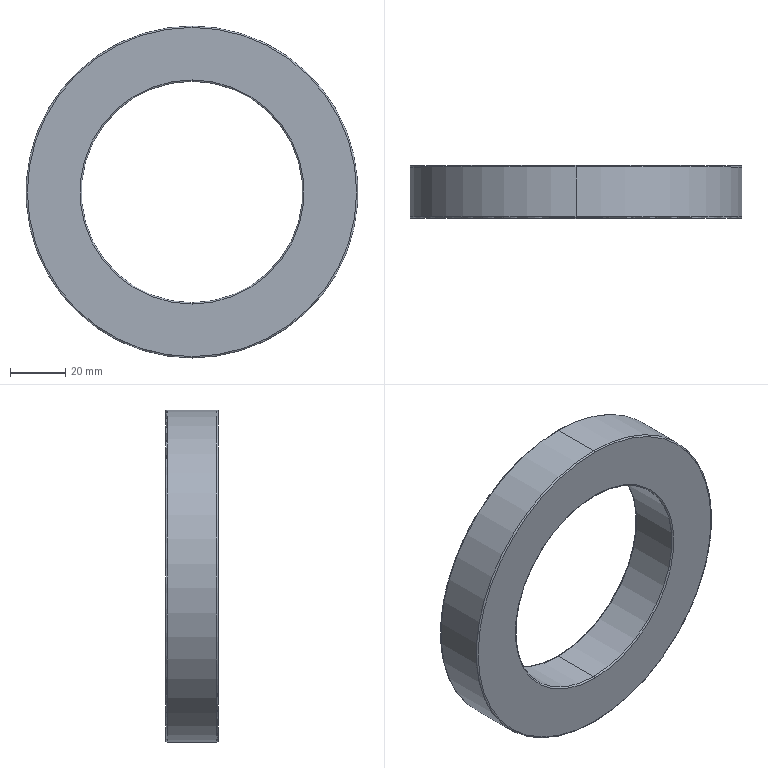Part | STEP file | 2026.6.15-Main Assembly图.sldasm-Part-126 | 1 solid | 14 faces | box 120 x 19 x 120 mm | volume 119313 mm3 | torus 8 | cylinder 4 | plane 2 | commonest cylinder face diameters 80 x2 120 x2
STEP:
#1=CARTESIAN_POINT('',(-1589.224,623.551,4168.167));
#2=VERTEX_POINT('',#1);
#3=CARTESIAN_POINT('',(-1589.224,623.551,4249.167));
#4=VERTEX_POINT('',#3);
#5=CARTESIAN_POINT('',(-1589.224,623.551,4208.667));
#6=DIRECTION('',(0.,-1.,0.));
#7=DIRECTION('',(0.,0.,1.));
#8=AXIS2_PLACEMENT_3D('',#5,#6,#7);
#9=CIRCLE('',#8,40.5);
#10=EDGE_CURVE('',#2,#4,#9,.T.);
#11=ORIENTED_EDGE('',*,*,#10,.F.);
#12=CARTESIAN_POINT('',(-1589.224,623.051,4168.667));
#13=VERTEX_POINT('',#12);
#14=CARTESIAN_POINT('',(-1589.224,623.051,4168.167));
#15=DIRECTION('',(1.,0.,0.));
#16=DIRECTION('',(0.,0.,-1.));
#17=AXIS2_PLACEMENT_3D('',#14,#15,#16);
#18=CIRCLE('',#17,0.5);
#19=EDGE_CURVE('',#2,#13,#18,.T.);
#20=ORIENTED_EDGE('',*,*,#19,.T.);
#21=CARTESIAN_POINT('',(-1589.224,623.051,4248.667));
#22=VERTEX_POINT('',#21);
#23=CARTESIAN_POINT('',(-1589.224,623.051,4208.667));
#24=DIRECTION('',(0.,1.,0.));
#25=DIRECTION('',(0.,0.,1.));
#26=AXIS2_PLACEMENT_3D('',#23,#24,#25);
#27=CIRCLE('',#26,40.);
#28=EDGE_CURVE('',#22,#13,#27,.T.);
#29=ORIENTED_EDGE('',*,*,#28,.F.);
#30=CARTESIAN_POINT('',(-1589.224,623.051,4249.167));
#31=DIRECTION('',(-1.,0.,0.));
#32=DIRECTION('',(0.,0.,1.));
#33=AXIS2_PLACEMENT_3D('',#30,#31,#32);
#34=CIRCLE('',#33,0.5);
#35=EDGE_CURVE('',#4,#22,#34,.T.);
#36=ORIENTED_EDGE('',*,*,#35,.F.);
#37=EDGE_LOOP('',(#11,#20,#29,#36));
#38=FACE_OUTER_BOUND('',#37,.T.);
#39=CARTESIAN_POINT('',(-1589.224,623.051,4208.667));
#40=DIRECTION('',(0.,1.,0.));
#41=DIRECTION('',(0.,0.,1.));
#42=AXIS2_PLACEMENT_3D('',#39,#40,#41);
#43=TOROIDAL_SURFACE('',#42,40.5,0.5);
#44=ADVANCED_FACE('',(#38),#43,.T.);
#45=CARTESIAN_POINT('',(-1589.224,623.051,4148.667));
#46=VERTEX_POINT('',#45);
#47=CARTESIAN_POINT('',(-1589.224,623.051,4268.667));
#48=VERTEX_POINT('',#47);
#49=CARTESIAN_POINT('',(-1589.224,623.051,4208.667));
#50=DIRECTION('',(0.,-1.,0.));
#51=DIRECTION('',(0.,0.,1.));
#52=AXIS2_PLACEMENT_3D('',#49,#50,#51);
#53=CIRCLE('',#52,60.);
#54=EDGE_CURVE('',#46,#48,#53,.T.);
#55=ORIENTED_EDGE('',*,*,#54,.F.);
#56=CARTESIAN_POINT('',(-1589.224,623.551,4149.167));
#57=VERTEX_POINT('',#56);
#58=CARTESIAN_POINT('',(-1589.224,623.051,4149.167));
#59=DIRECTION('',(1.,0.,0.));
#60=DIRECTION('',(0.,0.,-1.));
#61=AXIS2_PLACEMENT_3D('',#58,#59,#60);
#62=CIRCLE('',#61,0.5);
#63=EDGE_CURVE('',#46,#57,#62,.T.);
#64=ORIENTED_EDGE('',*,*,#63,.T.);
#65=CARTESIAN_POINT('',(-1589.224,623.551,4268.167));
#66=VERTEX_POINT('',#65);
#67=CARTESIAN_POINT('',(-1589.224,623.551,4208.667));
#68=DIRECTION('',(0.,1.,0.));
#69=DIRECTION('',(0.,0.,1.));
#70=AXIS2_PLACEMENT_3D('',#67,#68,#69);
#71=CIRCLE('',#70,59.5);
#72=EDGE_CURVE('',#66,#57,#71,.T.);
#73=ORIENTED_EDGE('',*,*,#72,.F.);
#74=CARTESIAN_POINT('',(-1589.224,623.051,4268.167));
#75=DIRECTION('',(-1.,0.,0.));
#76=DIRECTION('',(0.,0.,1.));
#77=AXIS2_PLACEMENT_3D('',#74,#75,#76);
#78=CIRCLE('',#77,0.5);
#79=EDGE_CURVE('',#48,#66,#78,.T.);
#80=ORIENTED_EDGE('',*,*,#79,.F.);
#81=EDGE_LOOP('',(#55,#64,#73,#80));
#82=FACE_OUTER_BOUND('',#81,.T.);
#83=CARTESIAN_POINT('',(-1589.224,623.051,4208.667));
#84=DIRECTION('',(0.,1.,0.));
#85=DIRECTION('',(0.,0.,1.));
#86=AXIS2_PLACEMENT_3D('',#83,#84,#85);
#87=TOROIDAL_SURFACE('',#86,59.5,0.5);
#88=ADVANCED_FACE('',(#82),#87,.T.);
#89=CARTESIAN_POINT('',(-1589.224,604.551,4249.167));
#90=VERTEX_POINT('',#89);
#91=CARTESIAN_POINT('',(-1589.224,604.551,4168.167));
#92=VERTEX_POINT('',#91);
#93=CARTESIAN_POINT('',(-1589.224,604.551,4208.667));
#94=DIRECTION('',(0.,1.,0.));
#95=DIRECTION('',(0.,0.,-1.));
#96=AXIS2_PLACEMENT_3D('',#93,#94,#95);
#97=CIRCLE('',#96,40.5);
#98=EDGE_CURVE('',#90,#92,#97,.T.);
#99=ORIENTED_EDGE('',*,*,#98,.F.);
#100=CARTESIAN_POINT('',(-1589.224,605.051,4248.667));
#101=VERTEX_POINT('',#100);
#102=CARTESIAN_POINT('',(-1589.224,605.051,4249.167));
#103=DIRECTION('',(1.,0.,0.));
#104=DIRECTION('',(0.,0.,-1.));
#105=AXIS2_PLACEMENT_3D('',#102,#103,#104);
#106=CIRCLE('',#105,0.5);
#107=EDGE_CURVE('',#90,#101,#106,.T.);
#108=ORIENTED_EDGE('',*,*,#107,.T.);
#109=CARTESIAN_POINT('',(-1589.224,605.051,4168.667));
#110=VERTEX_POINT('',#109);
#111=CARTESIAN_POINT('',(-1589.224,605.051,4208.667));
#112=DIRECTION('',(0.,-1.,0.));
#113=DIRECTION('',(0.,0.,-1.));
#114=AXIS2_PLACEMENT_3D('',#111,#112,#113);
#115=CIRCLE('',#114,40.);
#116=EDGE_CURVE('',#110,#101,#115,.T.);
#117=ORIENTED_EDGE('',*,*,#116,.F.);
#118=CARTESIAN_POINT('',(-1589.224,605.051,4168.167));
#119=DIRECTION('',(-1.,0.,0.));
#120=DIRECTION('',(0.,0.,1.));
#121=AXIS2_PLACEMENT_3D('',#118,#119,#120);
#122=CIRCLE('',#121,0.5);
#123=EDGE_CURVE('',#92,#110,#122,.T.);
#124=ORIENTED_EDGE('',*,*,#123,.F.);
#125=EDGE_LOOP('',(#99,#108,#117,#124));
#126=FACE_OUTER_BOUND('',#125,.T.);
#127=CARTESIAN_POINT('',(-1589.224,605.051,4208.667));
#128=DIRECTION('',(0.,-1.,0.));
#129=DIRECTION('',(0.,0.,-1.));
#130=AXIS2_PLACEMENT_3D('',#127,#128,#129);
#131=TOROIDAL_SURFACE('',#130,40.5,0.5);
#132=ADVANCED_FACE('',(#126),#131,.T.);
#133=CARTESIAN_POINT('',(-1589.224,605.051,4268.667));
#134=VERTEX_POINT('',#133);
#135=CARTESIAN_POINT('',(-1589.224,605.051,4148.667));
#136=VERTEX_POINT('',#135);
#137=CARTESIAN_POINT('',(-1589.224,605.051,4208.667));
#138=DIRECTION('',(0.,1.,0.));
#139=DIRECTION('',(0.,0.,-1.));
#140=AXIS2_PLACEMENT_3D('',#137,#138,#139);
#141=CIRCLE('',#140,60.);
#142=EDGE_CURVE('',#134,#136,#141,.T.);
#143=ORIENTED_EDGE('',*,*,#142,.F.);
#144=CARTESIAN_POINT('',(-1589.224,604.551,4268.167));
#145=VERTEX_POINT('',#144);
#146=CARTESIAN_POINT('',(-1589.224,605.051,4268.167));
#147=DIRECTION('',(1.,0.,0.));
#148=DIRECTION('',(0.,0.,-1.));
#149=AXIS2_PLACEMENT_3D('',#146,#147,#148);
#150=CIRCLE('',#149,0.5);
#151=EDGE_CURVE('',#134,#145,#150,.T.);
#152=ORIENTED_EDGE('',*,*,#151,.T.);
#153=CARTESIAN_POINT('',(-1589.224,604.551,4149.167));
#154=VERTEX_POINT('',#153);
#155=CARTESIAN_POINT('',(-1589.224,604.551,4208.667));
#156=DIRECTION('',(0.,-1.,0.));
#157=DIRECTION('',(0.,0.,-1.));
#158=AXIS2_PLACEMENT_3D('',#155,#156,#157);
#159=CIRCLE('',#158,59.5);
#160=EDGE_CURVE('',#154,#145,#159,.T.);
#161=ORIENTED_EDGE('',*,*,#160,.F.);
#162=CARTESIAN_POINT('',(-1589.224,605.051,4149.167));
#163=DIRECTION('',(-1.,0.,0.));
#164=DIRECTION('',(0.,0.,1.));
#165=AXIS2_PLACEMENT_3D('',#162,#163,#164);
#166=CIRCLE('',#165,0.5);
#167=EDGE_CURVE('',#136,#154,#166,.T.);
#168=ORIENTED_EDGE('',*,*,#167,.F.);
#169=EDGE_LOOP('',(#143,#152,#161,#168));
#170=FACE_OUTER_BOUND('',#169,.T.);
#171=CARTESIAN_POINT('',(-1589.224,605.051,4208.667));
#172=DIRECTION('',(0.,-1.,0.));
#173=DIRECTION('',(0.,0.,-1.));
#174=AXIS2_PLACEMENT_3D('',#171,#172,#173);
#175=TOROIDAL_SURFACE('',#174,59.5,0.5);
#176=ADVANCED_FACE('',(#170),#175,.T.);
#177=CARTESIAN_POINT('',(-1589.224,623.051,4208.667));
#178=DIRECTION('',(0.,1.,0.));
#179=DIRECTION('',(0.,0.,1.));
#180=AXIS2_PLACEMENT_3D('',#177,#178,#179);
#181=CIRCLE('',#180,40.);
#182=EDGE_CURVE('',#13,#22,#181,.T.);
#183=ORIENTED_EDGE('',*,*,#182,.T.);
#184=CARTESIAN_POINT('',(-1589.224,623.551,4248.667));
#185=DIRECTION('',(0.,-1.,0.));
#186=VECTOR('',#185,1000.);
#187=LINE('',#184,#186);
#188=EDGE_CURVE('',#22,#101,#187,.T.);
#189=ORIENTED_EDGE('',*,*,#188,.T.);
#190=CARTESIAN_POINT('',(-1589.224,605.051,4208.667));
#191=DIRECTION('',(0.,-1.,0.));
#192=DIRECTION('',(0.,0.,-1.));
#193=AXIS2_PLACEMENT_3D('',#190,#191,#192);
#194=CIRCLE('',#193,40.);
#195=EDGE_CURVE('',#101,#110,#194,.T.);
#196=ORIENTED_EDGE('',*,*,#195,.T.);
#197=CARTESIAN_POINT('',(-1589.224,623.551,4168.667));
#198=DIRECTION('',(0.,-1.,0.));
#199=VECTOR('',#198,1000.);
#200=LINE('',#197,#199);
#201=EDGE_CURVE('',#13,#110,#200,.T.);
#202=ORIENTED_EDGE('',*,*,#201,.F.);
#203=EDGE_LOOP('',(#183,#189,#196,#202));
#204=FACE_OUTER_BOUND('',#203,.T.);
#205=CARTESIAN_POINT('',(-1589.224,623.551,4208.667));
#206=DIRECTION('',(0.,-1.,0.));
#207=DIRECTION('',(0.,0.,-1.));
#208=AXIS2_PLACEMENT_3D('',#205,#206,#207);
#209=CYLINDRICAL_SURFACE('',#208,40.);
#210=ADVANCED_FACE('',(#204),#209,.F.);
#211=ORIENTED_EDGE('',*,*,#142,.T.);
#212=CARTESIAN_POINT('',(-1589.224,604.551,4148.667));
#213=DIRECTION('',(0.,1.,0.));
#214=VECTOR('',#213,1000.);
#215=LINE('',#212,#214);
#216=EDGE_CURVE('',#136,#46,#215,.T.);
#217=ORIENTED_EDGE('',*,*,#216,.T.);
#218=ORIENTED_EDGE('',*,*,#54,.T.);
#219=CARTESIAN_POINT('',(-1589.224,604.551,4268.667));
#220=DIRECTION('',(0.,1.,0.));
#221=VECTOR('',#220,1000.);
#222=LINE('',#219,#221);
#223=EDGE_CURVE('',#134,#48,#222,.T.);
#224=ORIENTED_EDGE('',*,*,#223,.F.);
#225=EDGE_LOOP('',(#211,#217,#218,#224));
#226=FACE_OUTER_BOUND('',#225,.T.);
#227=CARTESIAN_POINT('',(-1589.224,604.551,4208.667));
#228=DIRECTION('',(0.,1.,0.));
#229=DIRECTION('',(0.,0.,1.));
#230=AXIS2_PLACEMENT_3D('',#227,#228,#229);
#231=CYLINDRICAL_SURFACE('',#230,60.);
#232=ADVANCED_FACE('',(#226),#231,.T.);
#233=ORIENTED_EDGE('',*,*,#72,.T.);
#234=CARTESIAN_POINT('',(-1589.224,623.551,4208.667));
#235=DIRECTION('',(0.,1.,0.));
#236=DIRECTION('',(0.,0.,1.));
#237=AXIS2_PLACEMENT_3D('',#234,#235,#236);
#238=CIRCLE('',#237,59.5);
#239=EDGE_CURVE('',#57,#66,#238,.T.);
#240=ORIENTED_EDGE('',*,*,#239,.T.);
#241=EDGE_LOOP('',(#233,#240));
#242=FACE_OUTER_BOUND('',#241,.T.);
#243=CARTESIAN_POINT('',(-1589.224,623.551,4208.667));
#244=DIRECTION('',(0.,-1.,0.));
#245=DIRECTION('',(0.,0.,1.));
#246=AXIS2_PLACEMENT_3D('',#243,#244,#245);
#247=CIRCLE('',#246,40.5);
#248=EDGE_CURVE('',#4,#2,#247,.T.);
#249=ORIENTED_EDGE('',*,*,#248,.T.);
#250=ORIENTED_EDGE('',*,*,#10,.T.);
#251=EDGE_LOOP('',(#249,#250));
#252=FACE_BOUND('',#251,.T.);
#253=CARTESIAN_POINT('',(-1589.224,623.551,4208.667));
#254=DIRECTION('',(0.,1.,0.));
#255=DIRECTION('',(0.,0.,1.));
#256=AXIS2_PLACEMENT_3D('',#253,#254,#255);
#257=PLANE('',#256);
#258=ADVANCED_FACE('',(#242,#252),#257,.T.);
#259=ORIENTED_EDGE('',*,*,#160,.T.);
#260=CARTESIAN_POINT('',(-1589.224,604.551,4208.667));
#261=DIRECTION('',(0.,-1.,0.));
#262=DIRECTION('',(0.,0.,-1.));
#263=AXIS2_PLACEMENT_3D('',#260,#261,#262);
#264=CIRCLE('',#263,59.5);
#265=EDGE_CURVE('',#145,#154,#264,.T.);
#266=ORIENTED_EDGE('',*,*,#265,.T.);
#267=EDGE_LOOP('',(#259,#266));
#268=FACE_OUTER_BOUND('',#267,.T.);
#269=CARTESIAN_POINT('',(-1589.224,604.551,4208.667));
#270=DIRECTION('',(0.,1.,0.));
#271=DIRECTION('',(0.,0.,-1.));
#272=AXIS2_PLACEMENT_3D('',#269,#270,#271);
#273=CIRCLE('',#272,40.5);
#274=EDGE_CURVE('',#92,#90,#273,.T.);
#275=ORIENTED_EDGE('',*,*,#274,.T.);
#276=ORIENTED_EDGE('',*,*,#98,.T.);
#277=EDGE_LOOP('',(#275,#276));
#278=FACE_BOUND('',#277,.T.);
#279=CARTESIAN_POINT('',(-1589.224,604.551,4208.667));
#280=DIRECTION('',(0.,-1.,0.));
#281=DIRECTION('',(0.,0.,-1.));
#282=AXIS2_PLACEMENT_3D('',#279,#280,#281);
#283=PLANE('',#282);
#284=ADVANCED_FACE('',(#268,#278),#283,.T.);
#285=ORIENTED_EDGE('',*,*,#216,.F.);
#286=CARTESIAN_POINT('',(-1589.224,605.051,4208.667));
#287=DIRECTION('',(0.,1.,0.));
#288=DIRECTION('',(0.,0.,-1.));
#289=AXIS2_PLACEMENT_3D('',#286,#287,#288);
#290=CIRCLE('',#289,60.);
#291=EDGE_CURVE('',#136,#134,#290,.T.);
#292=ORIENTED_EDGE('',*,*,#291,.T.);
#293=ORIENTED_EDGE('',*,*,#223,.T.);
#294=CARTESIAN_POINT('',(-1589.224,623.051,4208.667));
#295=DIRECTION('',(0.,-1.,0.));
#296=DIRECTION('',(0.,0.,1.));
#297=AXIS2_PLACEMENT_3D('',#294,#295,#296);
#298=CIRCLE('',#297,60.);
#299=EDGE_CURVE('',#48,#46,#298,.T.);
#300=ORIENTED_EDGE('',*,*,#299,.T.);
#301=EDGE_LOOP('',(#285,#292,#293,#300));
#302=FACE_OUTER_BOUND('',#301,.T.);
#303=CARTESIAN_POINT('',(-1589.224,604.551,4208.667));
#304=DIRECTION('',(0.,1.,0.));
#305=DIRECTION('',(0.,0.,1.));
#306=AXIS2_PLACEMENT_3D('',#303,#304,#305);
#307=CYLINDRICAL_SURFACE('',#306,60.);
#308=ADVANCED_FACE('',(#302),#307,.T.);
#309=ORIENTED_EDGE('',*,*,#188,.F.);
#310=ORIENTED_EDGE('',*,*,#28,.T.);
#311=ORIENTED_EDGE('',*,*,#201,.T.);
#312=ORIENTED_EDGE('',*,*,#116,.T.);
#313=EDGE_LOOP('',(#309,#310,#311,#312));
#314=FACE_OUTER_BOUND('',#313,.T.);
#315=CARTESIAN_POINT('',(-1589.224,623.551,4208.667));
#316=DIRECTION('',(0.,-1.,0.));
#317=DIRECTION('',(0.,0.,-1.));
#318=AXIS2_PLACEMENT_3D('',#315,#316,#317);
#319=CYLINDRICAL_SURFACE('',#318,40.);
#320=ADVANCED_FACE('',(#314),#319,.F.);
#321=ORIENTED_EDGE('',*,*,#151,.F.);
#322=ORIENTED_EDGE('',*,*,#291,.F.);
#323=ORIENTED_EDGE('',*,*,#167,.T.);
#324=ORIENTED_EDGE('',*,*,#265,.F.);
#325=EDGE_LOOP('',(#321,#322,#323,#324));
#326=FACE_OUTER_BOUND('',#325,.T.);
#327=CARTESIAN_POINT('',(-1589.224,605.051,4208.667));
#328=DIRECTION('',(0.,-1.,0.));
#329=DIRECTION('',(0.,0.,-1.));
#330=AXIS2_PLACEMENT_3D('',#327,#328,#329);
#331=TOROIDAL_SURFACE('',#330,59.5,0.5);
#332=ADVANCED_FACE('',(#326),#331,.T.);
#333=ORIENTED_EDGE('',*,*,#107,.F.);
#334=ORIENTED_EDGE('',*,*,#274,.F.);
#335=ORIENTED_EDGE('',*,*,#123,.T.);
#336=ORIENTED_EDGE('',*,*,#195,.F.);
#337=EDGE_LOOP('',(#333,#334,#335,#336));
#338=FACE_OUTER_BOUND('',#337,.T.);
#339=CARTESIAN_POINT('',(-1589.224,605.051,4208.667));
#340=DIRECTION('',(0.,-1.,0.));
#341=DIRECTION('',(0.,0.,-1.));
#342=AXIS2_PLACEMENT_3D('',#339,#340,#341);
#343=TOROIDAL_SURFACE('',#342,40.5,0.5);
#344=ADVANCED_FACE('',(#338),#343,.T.);
#345=ORIENTED_EDGE('',*,*,#63,.F.);
#346=ORIENTED_EDGE('',*,*,#299,.F.);
#347=ORIENTED_EDGE('',*,*,#79,.T.);
#348=ORIENTED_EDGE('',*,*,#239,.F.);
#349=EDGE_LOOP('',(#345,#346,#347,#348));
#350=FACE_OUTER_BOUND('',#349,.T.);
#351=CARTESIAN_POINT('',(-1589.224,623.051,4208.667));
#352=DIRECTION('',(0.,1.,0.));
#353=DIRECTION('',(0.,0.,1.));
#354=AXIS2_PLACEMENT_3D('',#351,#352,#353);
#355=TOROIDAL_SURFACE('',#354,59.5,0.5);
#356=ADVANCED_FACE('',(#350),#355,.T.);
#357=ORIENTED_EDGE('',*,*,#19,.F.);
#358=ORIENTED_EDGE('',*,*,#248,.F.);
#359=ORIENTED_EDGE('',*,*,#35,.T.);
#360=ORIENTED_EDGE('',*,*,#182,.F.);
#361=EDGE_LOOP('',(#357,#358,#359,#360));
#362=FACE_OUTER_BOUND('',#361,.T.);
#363=CARTESIAN_POINT('',(-1589.224,623.051,4208.667));
#364=DIRECTION('',(0.,1.,0.));
#365=DIRECTION('',(0.,0.,1.));
#366=AXIS2_PLACEMENT_3D('',#363,#364,#365);
#367=TOROIDAL_SURFACE('',#366,40.5,0.5);
#368=ADVANCED_FACE('',(#362),#367,.T.);
#369=CLOSED_SHELL('',(#44,#88,#132,#176,#210,#232,#258,#284,#308,#320,#332,#344,#356,#368));
#370=MANIFOLD_SOLID_BREP('',#369);
#371=CARTESIAN_POINT('',(0.,0.,0.));
#372=DIRECTION('',(0.,0.,1.));
#373=DIRECTION('',(1.,0.,0.));
#374=AXIS2_PLACEMENT_3D('',#371,#372,#373);
#375=(LENGTH_UNIT()NAMED_UNIT(*)SI_UNIT(.MILLI.,.METRE.));
#376=UNCERTAINTY_MEASURE_WITH_UNIT(LENGTH_MEASURE(0.00001),#375,'','');
#377=(NAMED_UNIT(*)PLANE_ANGLE_UNIT()SI_UNIT($,.RADIAN.));
#378=(NAMED_UNIT(*)SI_UNIT($,.STERADIAN.)SOLID_ANGLE_UNIT());
#379=(GEOMETRIC_REPRESENTATION_CONTEXT(3)GLOBAL_UNCERTAINTY_ASSIGNED_CONTEXT((#376))GLOBAL_UNIT_ASSIGNED_CONTEXT((#375,#377,#378))REPRESENTATION_CONTEXT('',''));
#380=ADVANCED_BREP_SHAPE_REPRESENTATION('',(#370,#374),#379);